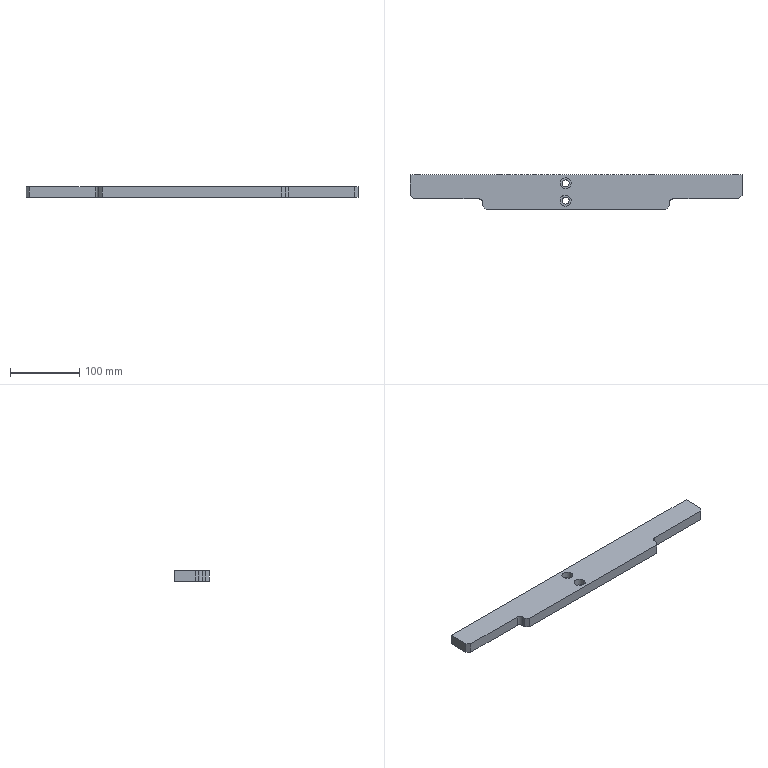Part | STEP file | J452-EBZ05-20-04-Part-1 | 1 solid | 54 faces | box 480 x 50 x 15 mm | volume 302912 mm3 | cylinder 26 | plane 20 | cone 8 | commonest cylinder face diameters 6.9 x8 8 x8 10 x6 16 x4